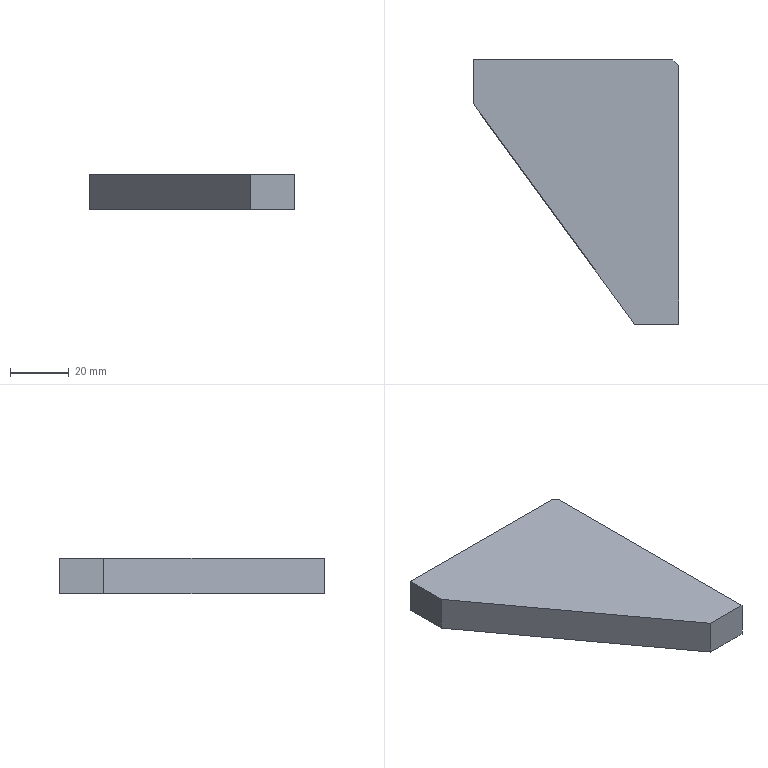Part | SolidWorks | features HoleWzd 2, Chamfer 1, Extrusion 1 | 1 solid | 24 faces | box 70 x 90 x 12 mm | volume 50116 mm3 | cylinder 8 | cone 8 | plane 8 | commonest cylinder face diameters 4.2 x8
STEP:
#1=CARTESIAN_POINT('',(-12.4,-75.,8.1));
#2=VERTEX_POINT('',#1);
#3=CARTESIAN_POINT('',(-12.4,-75.,3.9));
#4=VERTEX_POINT('',#3);
#5=CARTESIAN_POINT('',(-12.4,-75.,6.));
#6=DIRECTION('',(1.,0.,0.));
#7=DIRECTION('',(0.,0.,-1.));
#8=AXIS2_PLACEMENT_3D('',#5,#6,#7);
#9=CIRCLE('',#8,2.1);
#10=EDGE_CURVE('',#2,#4,#9,.T.);
#11=ORIENTED_EDGE('',*,*,#10,.F.);
#12=CARTESIAN_POINT('',(0.,-75.,8.1));
#13=VERTEX_POINT('',#12);
#14=CARTESIAN_POINT('',(0.,-75.,8.1));
#15=DIRECTION('',(1.,0.,0.));
#16=VECTOR('',#15,1000.);
#17=LINE('',#14,#16);
#18=EDGE_CURVE('',#2,#13,#17,.T.);
#19=ORIENTED_EDGE('',*,*,#18,.T.);
#20=CARTESIAN_POINT('',(0.,-75.,3.9));
#21=VERTEX_POINT('',#20);
#22=CARTESIAN_POINT('',(0.,-75.,6.));
#23=DIRECTION('',(1.,0.,0.));
#24=DIRECTION('',(0.,0.,-1.));
#25=AXIS2_PLACEMENT_3D('',#22,#23,#24);
#26=CIRCLE('',#25,2.1);
#27=EDGE_CURVE('',#13,#21,#26,.T.);
#28=ORIENTED_EDGE('',*,*,#27,.T.);
#29=CARTESIAN_POINT('',(0.,-75.,3.9));
#30=DIRECTION('',(1.,0.,0.));
#31=VECTOR('',#30,1000.);
#32=LINE('',#29,#31);
#33=EDGE_CURVE('',#4,#21,#32,.T.);
#34=ORIENTED_EDGE('',*,*,#33,.F.);
#35=EDGE_LOOP('',(#11,#19,#28,#34));
#36=FACE_OUTER_BOUND('',#35,.T.);
#37=CARTESIAN_POINT('',(0.,-75.,6.));
#38=DIRECTION('',(1.,0.,0.));
#39=DIRECTION('',(0.,0.,-1.));
#40=AXIS2_PLACEMENT_3D('',#37,#38,#39);
#41=CYLINDRICAL_SURFACE('',#40,2.1);
#42=ADVANCED_FACE('',(#36),#41,.F.);
#43=CARTESIAN_POINT('',(-13.662,-75.,6.));
#44=VERTEX_POINT('',#43);
#45=CARTESIAN_POINT('',(-12.4,-75.,3.9));
#46=DIRECTION('',(0.515,0.,-0.8572));
#47=VECTOR('',#46,1000.);
#48=LINE('',#45,#47);
#49=EDGE_CURVE('',#44,#4,#48,.T.);
#50=ORIENTED_EDGE('',*,*,#49,.F.);
#51=CARTESIAN_POINT('',(-12.4,-75.,8.1));
#52=DIRECTION('',(0.515,0.,0.8572));
#53=VECTOR('',#52,1000.);
#54=LINE('',#51,#53);
#55=EDGE_CURVE('',#44,#2,#54,.T.);
#56=ORIENTED_EDGE('',*,*,#55,.T.);
#57=ORIENTED_EDGE('',*,*,#10,.T.);
#58=EDGE_LOOP('',(#50,#56,#57));
#59=FACE_OUTER_BOUND('',#58,.T.);
#60=CARTESIAN_POINT('',(-12.4,-75.,6.));
#61=DIRECTION('',(1.,0.,0.));
#62=DIRECTION('',(0.,0.,-1.));
#63=AXIS2_PLACEMENT_3D('',#60,#61,#62);
#64=CONICAL_SURFACE('',#63,2.1,1.03);
#65=ADVANCED_FACE('',(#59),#64,.F.);
#66=CARTESIAN_POINT('',(-12.4,-25.,8.1));
#67=VERTEX_POINT('',#66);
#68=CARTESIAN_POINT('',(-12.4,-25.,3.9));
#69=VERTEX_POINT('',#68);
#70=CARTESIAN_POINT('',(-12.4,-25.,6.));
#71=DIRECTION('',(1.,0.,0.));
#72=DIRECTION('',(0.,0.,-1.));
#73=AXIS2_PLACEMENT_3D('',#70,#71,#72);
#74=CIRCLE('',#73,2.1);
#75=EDGE_CURVE('',#67,#69,#74,.T.);
#76=ORIENTED_EDGE('',*,*,#75,.F.);
#77=CARTESIAN_POINT('',(0.,-25.,8.1));
#78=VERTEX_POINT('',#77);
#79=CARTESIAN_POINT('',(0.,-25.,8.1));
#80=DIRECTION('',(1.,0.,0.));
#81=VECTOR('',#80,1000.);
#82=LINE('',#79,#81);
#83=EDGE_CURVE('',#67,#78,#82,.T.);
#84=ORIENTED_EDGE('',*,*,#83,.T.);
#85=CARTESIAN_POINT('',(0.,-25.,3.9));
#86=VERTEX_POINT('',#85);
#87=CARTESIAN_POINT('',(0.,-25.,6.));
#88=DIRECTION('',(1.,0.,0.));
#89=DIRECTION('',(0.,0.,-1.));
#90=AXIS2_PLACEMENT_3D('',#87,#88,#89);
#91=CIRCLE('',#90,2.1);
#92=EDGE_CURVE('',#78,#86,#91,.T.);
#93=ORIENTED_EDGE('',*,*,#92,.T.);
#94=CARTESIAN_POINT('',(0.,-25.,3.9));
#95=DIRECTION('',(1.,0.,0.));
#96=VECTOR('',#95,1000.);
#97=LINE('',#94,#96);
#98=EDGE_CURVE('',#69,#86,#97,.T.);
#99=ORIENTED_EDGE('',*,*,#98,.F.);
#100=EDGE_LOOP('',(#76,#84,#93,#99));
#101=FACE_OUTER_BOUND('',#100,.T.);
#102=CARTESIAN_POINT('',(0.,-25.,6.));
#103=DIRECTION('',(1.,0.,0.));
#104=DIRECTION('',(0.,0.,-1.));
#105=AXIS2_PLACEMENT_3D('',#102,#103,#104);
#106=CYLINDRICAL_SURFACE('',#105,2.1);
#107=ADVANCED_FACE('',(#101),#106,.F.);
#108=CARTESIAN_POINT('',(-13.662,-25.,6.));
#109=VERTEX_POINT('',#108);
#110=CARTESIAN_POINT('',(-12.4,-25.,3.9));
#111=DIRECTION('',(0.515,0.,-0.8572));
#112=VECTOR('',#111,1000.);
#113=LINE('',#110,#112);
#114=EDGE_CURVE('',#109,#69,#113,.T.);
#115=ORIENTED_EDGE('',*,*,#114,.F.);
#116=CARTESIAN_POINT('',(-12.4,-25.,8.1));
#117=DIRECTION('',(0.515,0.,0.8572));
#118=VECTOR('',#117,1000.);
#119=LINE('',#116,#118);
#120=EDGE_CURVE('',#109,#67,#119,.T.);
#121=ORIENTED_EDGE('',*,*,#120,.T.);
#122=ORIENTED_EDGE('',*,*,#75,.T.);
#123=EDGE_LOOP('',(#115,#121,#122));
#124=FACE_OUTER_BOUND('',#123,.T.);
#125=CARTESIAN_POINT('',(-12.4,-25.,6.));
#126=DIRECTION('',(1.,0.,0.));
#127=DIRECTION('',(0.,0.,-1.));
#128=AXIS2_PLACEMENT_3D('',#125,#126,#127);
#129=CONICAL_SURFACE('',#128,2.1,1.03);
#130=ADVANCED_FACE('',(#124),#129,.F.);
#131=CARTESIAN_POINT('',(-60.,-12.4,3.9));
#132=VERTEX_POINT('',#131);
#133=CARTESIAN_POINT('',(-60.,-12.4,8.1));
#134=VERTEX_POINT('',#133);
#135=CARTESIAN_POINT('',(-60.,-12.4,6.));
#136=DIRECTION('',(0.,1.,0.));
#137=DIRECTION('',(0.,0.,1.));
#138=AXIS2_PLACEMENT_3D('',#135,#136,#137);
#139=CIRCLE('',#138,2.1);
#140=EDGE_CURVE('',#132,#134,#139,.T.);
#141=ORIENTED_EDGE('',*,*,#140,.F.);
#142=CARTESIAN_POINT('',(-60.,0.,3.9));
#143=VERTEX_POINT('',#142);
#144=CARTESIAN_POINT('',(-60.,0.,3.9));
#145=DIRECTION('',(0.,1.,0.));
#146=VECTOR('',#145,1000.);
#147=LINE('',#144,#146);
#148=EDGE_CURVE('',#132,#143,#147,.T.);
#149=ORIENTED_EDGE('',*,*,#148,.T.);
#150=CARTESIAN_POINT('',(-60.,0.,8.1));
#151=VERTEX_POINT('',#150);
#152=CARTESIAN_POINT('',(-60.,0.,6.));
#153=DIRECTION('',(0.,1.,0.));
#154=DIRECTION('',(0.,0.,1.));
#155=AXIS2_PLACEMENT_3D('',#152,#153,#154);
#156=CIRCLE('',#155,2.1);
#157=EDGE_CURVE('',#143,#151,#156,.T.);
#158=ORIENTED_EDGE('',*,*,#157,.T.);
#159=CARTESIAN_POINT('',(-60.,0.,8.1));
#160=DIRECTION('',(0.,1.,0.));
#161=VECTOR('',#160,1000.);
#162=LINE('',#159,#161);
#163=EDGE_CURVE('',#134,#151,#162,.T.);
#164=ORIENTED_EDGE('',*,*,#163,.F.);
#165=EDGE_LOOP('',(#141,#149,#158,#164));
#166=FACE_OUTER_BOUND('',#165,.T.);
#167=CARTESIAN_POINT('',(-60.,0.,6.));
#168=DIRECTION('',(0.,1.,0.));
#169=DIRECTION('',(0.,0.,1.));
#170=AXIS2_PLACEMENT_3D('',#167,#168,#169);
#171=CYLINDRICAL_SURFACE('',#170,2.1);
#172=ADVANCED_FACE('',(#166),#171,.F.);
#173=CARTESIAN_POINT('',(-60.,-13.662,6.));
#174=VERTEX_POINT('',#173);
#175=CARTESIAN_POINT('',(-60.,-12.4,8.1));
#176=DIRECTION('',(0.,0.515,0.8572));
#177=VECTOR('',#176,1000.);
#178=LINE('',#175,#177);
#179=EDGE_CURVE('',#174,#134,#178,.T.);
#180=ORIENTED_EDGE('',*,*,#179,.F.);
#181=CARTESIAN_POINT('',(-60.,-12.4,3.9));
#182=DIRECTION('',(0.,0.515,-0.8572));
#183=VECTOR('',#182,1000.);
#184=LINE('',#181,#183);
#185=EDGE_CURVE('',#174,#132,#184,.T.);
#186=ORIENTED_EDGE('',*,*,#185,.T.);
#187=ORIENTED_EDGE('',*,*,#140,.T.);
#188=EDGE_LOOP('',(#180,#186,#187));
#189=FACE_OUTER_BOUND('',#188,.T.);
#190=CARTESIAN_POINT('',(-60.,-12.4,6.));
#191=DIRECTION('',(0.,1.,0.));
#192=DIRECTION('',(0.,0.,1.));
#193=AXIS2_PLACEMENT_3D('',#190,#191,#192);
#194=CONICAL_SURFACE('',#193,2.1,1.03);
#195=ADVANCED_FACE('',(#189),#194,.F.);
#196=CARTESIAN_POINT('',(-30.,-12.4,3.9));
#197=VERTEX_POINT('',#196);
#198=CARTESIAN_POINT('',(-30.,-12.4,8.1));
#199=VERTEX_POINT('',#198);
#200=CARTESIAN_POINT('',(-30.,-12.4,6.));
#201=DIRECTION('',(0.,1.,0.));
#202=DIRECTION('',(0.,0.,1.));
#203=AXIS2_PLACEMENT_3D('',#200,#201,#202);
#204=CIRCLE('',#203,2.1);
#205=EDGE_CURVE('',#197,#199,#204,.T.);
#206=ORIENTED_EDGE('',*,*,#205,.F.);
#207=CARTESIAN_POINT('',(-30.,0.,3.9));
#208=VERTEX_POINT('',#207);
#209=CARTESIAN_POINT('',(-30.,0.,3.9));
#210=DIRECTION('',(0.,1.,0.));
#211=VECTOR('',#210,1000.);
#212=LINE('',#209,#211);
#213=EDGE_CURVE('',#197,#208,#212,.T.);
#214=ORIENTED_EDGE('',*,*,#213,.T.);
#215=CARTESIAN_POINT('',(-30.,0.,8.1));
#216=VERTEX_POINT('',#215);
#217=CARTESIAN_POINT('',(-30.,0.,6.));
#218=DIRECTION('',(0.,1.,0.));
#219=DIRECTION('',(0.,0.,1.));
#220=AXIS2_PLACEMENT_3D('',#217,#218,#219);
#221=CIRCLE('',#220,2.1);
#222=EDGE_CURVE('',#208,#216,#221,.T.);
#223=ORIENTED_EDGE('',*,*,#222,.T.);
#224=CARTESIAN_POINT('',(-30.,0.,8.1));
#225=DIRECTION('',(0.,1.,0.));
#226=VECTOR('',#225,1000.);
#227=LINE('',#224,#226);
#228=EDGE_CURVE('',#199,#216,#227,.T.);
#229=ORIENTED_EDGE('',*,*,#228,.F.);
#230=EDGE_LOOP('',(#206,#214,#223,#229));
#231=FACE_OUTER_BOUND('',#230,.T.);
#232=CARTESIAN_POINT('',(-30.,0.,6.));
#233=DIRECTION('',(0.,1.,0.));
#234=DIRECTION('',(0.,0.,1.));
#235=AXIS2_PLACEMENT_3D('',#232,#233,#234);
#236=CYLINDRICAL_SURFACE('',#235,2.1);
#237=ADVANCED_FACE('',(#231),#236,.F.);
#238=CARTESIAN_POINT('',(-30.,-13.662,6.));
#239=VERTEX_POINT('',#238);
#240=CARTESIAN_POINT('',(-30.,-12.4,8.1));
#241=DIRECTION('',(0.,0.515,0.8572));
#242=VECTOR('',#241,1000.);
#243=LINE('',#240,#242);
#244=EDGE_CURVE('',#239,#199,#243,.T.);
#245=ORIENTED_EDGE('',*,*,#244,.F.);
#246=CARTESIAN_POINT('',(-30.,-12.4,3.9));
#247=DIRECTION('',(0.,0.515,-0.8572));
#248=VECTOR('',#247,1000.);
#249=LINE('',#246,#248);
#250=EDGE_CURVE('',#239,#197,#249,.T.);
#251=ORIENTED_EDGE('',*,*,#250,.T.);
#252=ORIENTED_EDGE('',*,*,#205,.T.);
#253=EDGE_LOOP('',(#245,#251,#252));
#254=FACE_OUTER_BOUND('',#253,.T.);
#255=CARTESIAN_POINT('',(-30.,-12.4,6.));
#256=DIRECTION('',(0.,1.,0.));
#257=DIRECTION('',(0.,0.,1.));
#258=AXIS2_PLACEMENT_3D('',#255,#256,#257);
#259=CONICAL_SURFACE('',#258,2.1,1.03);
#260=ADVANCED_FACE('',(#254),#259,.F.);
#261=CARTESIAN_POINT('',(-60.,0.,6.));
#262=DIRECTION('',(0.,1.,0.));
#263=DIRECTION('',(0.,0.,1.));
#264=AXIS2_PLACEMENT_3D('',#261,#262,#263);
#265=CIRCLE('',#264,2.1);
#266=EDGE_CURVE('',#151,#143,#265,.T.);
#267=ORIENTED_EDGE('',*,*,#266,.F.);
#268=ORIENTED_EDGE('',*,*,#157,.F.);
#269=EDGE_LOOP('',(#267,#268));
#270=FACE_BOUND('',#269,.T.);
#271=CARTESIAN_POINT('',(-30.,0.,6.));
#272=DIRECTION('',(0.,1.,0.));
#273=DIRECTION('',(0.,0.,1.));
#274=AXIS2_PLACEMENT_3D('',#271,#272,#273);
#275=CIRCLE('',#274,2.1);
#276=EDGE_CURVE('',#216,#208,#275,.T.);
#277=ORIENTED_EDGE('',*,*,#276,.F.);
#278=ORIENTED_EDGE('',*,*,#222,.F.);
#279=EDGE_LOOP('',(#277,#278));
#280=FACE_BOUND('',#279,.T.);
#281=CARTESIAN_POINT('',(-2.,0.,12.));
#282=VERTEX_POINT('',#281);
#283=CARTESIAN_POINT('',(-70.,0.,12.));
#284=VERTEX_POINT('',#283);
#285=CARTESIAN_POINT('',(-70.,0.,12.));
#286=DIRECTION('',(-1.,0.,0.));
#287=VECTOR('',#286,1000.);
#288=LINE('',#285,#287);
#289=EDGE_CURVE('',#282,#284,#288,.T.);
#290=ORIENTED_EDGE('',*,*,#289,.F.);
#291=CARTESIAN_POINT('',(-2.,0.,0.));
#292=VERTEX_POINT('',#291);
#293=CARTESIAN_POINT('',(-2.,0.,12.));
#294=DIRECTION('',(0.,0.,-1.));
#295=VECTOR('',#294,1000.);
#296=LINE('',#293,#295);
#297=EDGE_CURVE('',#282,#292,#296,.T.);
#298=ORIENTED_EDGE('',*,*,#297,.T.);
#299=CARTESIAN_POINT('',(-70.,0.,0.));
#300=VERTEX_POINT('',#299);
#301=CARTESIAN_POINT('',(-70.,0.,0.));
#302=DIRECTION('',(-1.,0.,0.));
#303=VECTOR('',#302,1000.);
#304=LINE('',#301,#303);
#305=EDGE_CURVE('',#292,#300,#304,.T.);
#306=ORIENTED_EDGE('',*,*,#305,.T.);
#307=CARTESIAN_POINT('',(-70.,0.,12.));
#308=DIRECTION('',(0.,0.,-1.));
#309=VECTOR('',#308,1000.);
#310=LINE('',#307,#309);
#311=EDGE_CURVE('',#284,#300,#310,.T.);
#312=ORIENTED_EDGE('',*,*,#311,.F.);
#313=EDGE_LOOP('',(#290,#298,#306,#312));
#314=FACE_OUTER_BOUND('',#313,.T.);
#315=CARTESIAN_POINT('',(-70.,0.,12.));
#316=DIRECTION('',(0.,-1.,0.));
#317=DIRECTION('',(0.,0.,-1.));
#318=AXIS2_PLACEMENT_3D('',#315,#316,#317);
#319=PLANE('',#318);
#320=ADVANCED_FACE('',(#270,#280,#314),#319,.F.);
#321=CARTESIAN_POINT('',(-70.,-15.,0.));
#322=VERTEX_POINT('',#321);
#323=CARTESIAN_POINT('',(-70.,-15.,0.));
#324=DIRECTION('',(0.,-1.,0.));
#325=VECTOR('',#324,1000.);
#326=LINE('',#323,#325);
#327=EDGE_CURVE('',#300,#322,#326,.T.);
#328=ORIENTED_EDGE('',*,*,#327,.T.);
#329=CARTESIAN_POINT('',(-70.,-15.,12.));
#330=VERTEX_POINT('',#329);
#331=CARTESIAN_POINT('',(-70.,-15.,12.));
#332=DIRECTION('',(0.,0.,-1.));
#333=VECTOR('',#332,1000.);
#334=LINE('',#331,#333);
#335=EDGE_CURVE('',#330,#322,#334,.T.);
#336=ORIENTED_EDGE('',*,*,#335,.F.);
#337=CARTESIAN_POINT('',(-70.,-15.,12.));
#338=DIRECTION('',(0.,-1.,0.));
#339=VECTOR('',#338,1000.);
#340=LINE('',#337,#339);
#341=EDGE_CURVE('',#284,#330,#340,.T.);
#342=ORIENTED_EDGE('',*,*,#341,.F.);
#343=ORIENTED_EDGE('',*,*,#311,.T.);
#344=EDGE_LOOP('',(#328,#336,#342,#343));
#345=FACE_OUTER_BOUND('',#344,.T.);
#346=CARTESIAN_POINT('',(-70.,-15.,12.));
#347=DIRECTION('',(1.,0.,0.));
#348=DIRECTION('',(0.,0.,-1.));
#349=AXIS2_PLACEMENT_3D('',#346,#347,#348);
#350=PLANE('',#349);
#351=ADVANCED_FACE('',(#345),#350,.F.);
#352=CARTESIAN_POINT('',(-15.,-90.,0.));
#353=VERTEX_POINT('',#352);
#354=CARTESIAN_POINT('',(-15.,-90.,0.));
#355=DIRECTION('',(0.5914,-0.8064,0.));
#356=VECTOR('',#355,1000.);
#357=LINE('',#354,#356);
#358=EDGE_CURVE('',#322,#353,#357,.T.);
#359=ORIENTED_EDGE('',*,*,#358,.T.);
#360=CARTESIAN_POINT('',(-15.,-90.,12.));
#361=VERTEX_POINT('',#360);
#362=CARTESIAN_POINT('',(-15.,-90.,12.));
#363=DIRECTION('',(0.,0.,-1.));
#364=VECTOR('',#363,1000.);
#365=LINE('',#362,#364);
#366=EDGE_CURVE('',#361,#353,#365,.T.);
#367=ORIENTED_EDGE('',*,*,#366,.F.);
#368=CARTESIAN_POINT('',(-15.,-90.,12.));
#369=DIRECTION('',(0.5914,-0.8064,0.));
#370=VECTOR('',#369,1000.);
#371=LINE('',#368,#370);
#372=EDGE_CURVE('',#330,#361,#371,.T.);
#373=ORIENTED_EDGE('',*,*,#372,.F.);
#374=ORIENTED_EDGE('',*,*,#335,.T.);
#375=EDGE_LOOP('',(#359,#367,#373,#374));
#376=FACE_OUTER_BOUND('',#375,.T.);
#377=CARTESIAN_POINT('',(-15.,-90.,12.));
#378=DIRECTION('',(0.8064,0.5914,0.));
#379=DIRECTION('',(-0.5914,0.8064,0.));
#380=AXIS2_PLACEMENT_3D('',#377,#378,#379);
#381=PLANE('',#380);
#382=ADVANCED_FACE('',(#376),#381,.F.);
#383=CARTESIAN_POINT('',(0.,-90.,0.));
#384=VERTEX_POINT('',#383);
#385=CARTESIAN_POINT('',(0.,-90.,0.));
#386=DIRECTION('',(1.,0.,0.));
#387=VECTOR('',#386,1000.);
#388=LINE('',#385,#387);
#389=EDGE_CURVE('',#353,#384,#388,.T.);
#390=ORIENTED_EDGE('',*,*,#389,.T.);
#391=CARTESIAN_POINT('',(0.,-90.,12.));
#392=VERTEX_POINT('',#391);
#393=CARTESIAN_POINT('',(0.,-90.,12.));
#394=DIRECTION('',(0.,0.,-1.));
#395=VECTOR('',#394,1000.);
#396=LINE('',#393,#395);
#397=EDGE_CURVE('',#392,#384,#396,.T.);
#398=ORIENTED_EDGE('',*,*,#397,.F.);
#399=CARTESIAN_POINT('',(0.,-90.,12.));
#400=DIRECTION('',(1.,0.,0.));
#401=VECTOR('',#400,1000.);
#402=LINE('',#399,#401);
#403=EDGE_CURVE('',#361,#392,#402,.T.);
#404=ORIENTED_EDGE('',*,*,#403,.F.);
#405=ORIENTED_EDGE('',*,*,#366,.T.);
#406=EDGE_LOOP('',(#390,#398,#404,#405));
#407=FACE_OUTER_BOUND('',#406,.T.);
#408=CARTESIAN_POINT('',(0.,-90.,12.));
#409=DIRECTION('',(0.,1.,0.));
#410=DIRECTION('',(0.,0.,1.));
#411=AXIS2_PLACEMENT_3D('',#408,#409,#410);
#412=PLANE('',#411);
#413=ADVANCED_FACE('',(#407),#412,.F.);
#414=CARTESIAN_POINT('',(0.,-75.,6.));
#415=DIRECTION('',(1.,0.,0.));
#416=DIRECTION('',(0.,0.,-1.));
#417=AXIS2_PLACEMENT_3D('',#414,#415,#416);
#418=CIRCLE('',#417,2.1);
#419=EDGE_CURVE('',#21,#13,#418,.T.);
#420=ORIENTED_EDGE('',*,*,#419,.F.);
#421=ORIENTED_EDGE('',*,*,#27,.F.);
#422=EDGE_LOOP('',(#420,#421));
#423=FACE_BOUND('',#422,.T.);
#424=CARTESIAN_POINT('',(0.,-25.,6.));
#425=DIRECTION('',(1.,0.,0.));
#426=DIRECTION('',(0.,0.,-1.));
#427=AXIS2_PLACEMENT_3D('',#424,#425,#426);
#428=CIRCLE('',#427,2.1);
#429=EDGE_CURVE('',#86,#78,#428,.T.);
#430=ORIENTED_EDGE('',*,*,#429,.F.);
#431=ORIENTED_EDGE('',*,*,#92,.F.);
#432=EDGE_LOOP('',(#430,#431));
#433=FACE_BOUND('',#432,.T.);
#434=CARTESIAN_POINT('',(0.,-2.,0.));
#435=VERTEX_POINT('',#434);
#436=CARTESIAN_POINT('',(0.,0.,0.));
#437=DIRECTION('',(0.,1.,0.));
#438=VECTOR('',#437,1000.);
#439=LINE('',#436,#438);
#440=EDGE_CURVE('',#384,#435,#439,.T.);
#441=ORIENTED_EDGE('',*,*,#440,.T.);
#442=CARTESIAN_POINT('',(0.,-2.,12.));
#443=VERTEX_POINT('',#442);
#444=CARTESIAN_POINT('',(0.,-2.,12.));
#445=DIRECTION('',(0.,0.,1.));
#446=VECTOR('',#445,1000.);
#447=LINE('',#444,#446);
#448=EDGE_CURVE('',#435,#443,#447,.T.);
#449=ORIENTED_EDGE('',*,*,#448,.T.);
#450=CARTESIAN_POINT('',(0.,0.,12.));
#451=DIRECTION('',(0.,1.,0.));
#452=VECTOR('',#451,1000.);
#453=LINE('',#450,#452);
#454=EDGE_CURVE('',#392,#443,#453,.T.);
#455=ORIENTED_EDGE('',*,*,#454,.F.);
#456=ORIENTED_EDGE('',*,*,#397,.T.);
#457=EDGE_LOOP('',(#441,#449,#455,#456));
#458=FACE_OUTER_BOUND('',#457,.T.);
#459=CARTESIAN_POINT('',(0.,0.,12.));
#460=DIRECTION('',(-1.,0.,0.));
#461=DIRECTION('',(0.,-1.,0.));
#462=AXIS2_PLACEMENT_3D('',#459,#460,#461);
#463=PLANE('',#462);
#464=ADVANCED_FACE('',(#423,#433,#458),#463,.F.);
#465=ORIENTED_EDGE('',*,*,#454,.T.);
#466=CARTESIAN_POINT('',(-2.,0.,12.));
#467=DIRECTION('',(-0.7071,0.7071,0.));
#468=VECTOR('',#467,1000.);
#469=LINE('',#466,#468);
#470=EDGE_CURVE('',#443,#282,#469,.T.);
#471=ORIENTED_EDGE('',*,*,#470,.T.);
#472=ORIENTED_EDGE('',*,*,#289,.T.);
#473=ORIENTED_EDGE('',*,*,#341,.T.);
#474=ORIENTED_EDGE('',*,*,#372,.T.);
#475=ORIENTED_EDGE('',*,*,#403,.T.);
#476=EDGE_LOOP('',(#465,#471,#472,#473,#474,#475));
#477=FACE_OUTER_BOUND('',#476,.T.);
#478=CARTESIAN_POINT('',(0.,0.,12.));
#479=DIRECTION('',(0.,0.,-1.));
#480=DIRECTION('',(-1.,0.,0.));
#481=AXIS2_PLACEMENT_3D('',#478,#479,#480);
#482=PLANE('',#481);
#483=ADVANCED_FACE('',(#477),#482,.F.);
#484=ORIENTED_EDGE('',*,*,#305,.F.);
#485=CARTESIAN_POINT('',(-1.,-1.,0.));
#486=DIRECTION('',(0.7071,-0.7071,0.));
#487=VECTOR('',#486,1000.);
#488=LINE('',#485,#487);
#489=EDGE_CURVE('',#292,#435,#488,.T.);
#490=ORIENTED_EDGE('',*,*,#489,.T.);
#491=ORIENTED_EDGE('',*,*,#440,.F.);
#492=ORIENTED_EDGE('',*,*,#389,.F.);
#493=ORIENTED_EDGE('',*,*,#358,.F.);
#494=ORIENTED_EDGE('',*,*,#327,.F.);
#495=EDGE_LOOP('',(#484,#490,#491,#492,#493,#494));
#496=FACE_OUTER_BOUND('',#495,.T.);
#497=CARTESIAN_POINT('',(0.,0.,0.));
#498=DIRECTION('',(0.,0.,-1.));
#499=DIRECTION('',(-1.,0.,0.));
#500=AXIS2_PLACEMENT_3D('',#497,#498,#499);
#501=PLANE('',#500);
#502=ADVANCED_FACE('',(#496),#501,.T.);
#503=ORIENTED_EDGE('',*,*,#250,.F.);
#504=ORIENTED_EDGE('',*,*,#244,.T.);
#505=CARTESIAN_POINT('',(-30.,-12.4,6.));
#506=DIRECTION('',(0.,1.,0.));
#507=DIRECTION('',(0.,0.,1.));
#508=AXIS2_PLACEMENT_3D('',#505,#506,#507);
#509=CIRCLE('',#508,2.1);
#510=EDGE_CURVE('',#199,#197,#509,.T.);
#511=ORIENTED_EDGE('',*,*,#510,.T.);
#512=EDGE_LOOP('',(#503,#504,#511));
#513=FACE_OUTER_BOUND('',#512,.T.);
#514=CARTESIAN_POINT('',(-30.,-12.4,6.));
#515=DIRECTION('',(0.,1.,0.));
#516=DIRECTION('',(0.,0.,1.));
#517=AXIS2_PLACEMENT_3D('',#514,#515,#516);
#518=CONICAL_SURFACE('',#517,2.1,1.03);
#519=ADVANCED_FACE('',(#513),#518,.F.);
#520=ORIENTED_EDGE('',*,*,#213,.F.);
#521=ORIENTED_EDGE('',*,*,#510,.F.);
#522=ORIENTED_EDGE('',*,*,#228,.T.);
#523=ORIENTED_EDGE('',*,*,#276,.T.);
#524=EDGE_LOOP('',(#520,#521,#522,#523));
#525=FACE_OUTER_BOUND('',#524,.T.);
#526=CARTESIAN_POINT('',(-30.,0.,6.));
#527=DIRECTION('',(0.,1.,0.));
#528=DIRECTION('',(0.,0.,1.));
#529=AXIS2_PLACEMENT_3D('',#526,#527,#528);
#530=CYLINDRICAL_SURFACE('',#529,2.1);
#531=ADVANCED_FACE('',(#525),#530,.F.);
#532=ORIENTED_EDGE('',*,*,#185,.F.);
#533=ORIENTED_EDGE('',*,*,#179,.T.);
#534=CARTESIAN_POINT('',(-60.,-12.4,6.));
#535=DIRECTION('',(0.,1.,0.));
#536=DIRECTION('',(0.,0.,1.));
#537=AXIS2_PLACEMENT_3D('',#534,#535,#536);
#538=CIRCLE('',#537,2.1);
#539=EDGE_CURVE('',#134,#132,#538,.T.);
#540=ORIENTED_EDGE('',*,*,#539,.T.);
#541=EDGE_LOOP('',(#532,#533,#540));
#542=FACE_OUTER_BOUND('',#541,.T.);
#543=CARTESIAN_POINT('',(-60.,-12.4,6.));
#544=DIRECTION('',(0.,1.,0.));
#545=DIRECTION('',(0.,0.,1.));
#546=AXIS2_PLACEMENT_3D('',#543,#544,#545);
#547=CONICAL_SURFACE('',#546,2.1,1.03);
#548=ADVANCED_FACE('',(#542),#547,.F.);
#549=ORIENTED_EDGE('',*,*,#148,.F.);
#550=ORIENTED_EDGE('',*,*,#539,.F.);
#551=ORIENTED_EDGE('',*,*,#163,.T.);
#552=ORIENTED_EDGE('',*,*,#266,.T.);
#553=EDGE_LOOP('',(#549,#550,#551,#552));
#554=FACE_OUTER_BOUND('',#553,.T.);
#555=CARTESIAN_POINT('',(-60.,0.,6.));
#556=DIRECTION('',(0.,1.,0.));
#557=DIRECTION('',(0.,0.,1.));
#558=AXIS2_PLACEMENT_3D('',#555,#556,#557);
#559=CYLINDRICAL_SURFACE('',#558,2.1);
#560=ADVANCED_FACE('',(#554),#559,.F.);
#561=ORIENTED_EDGE('',*,*,#120,.F.);
#562=ORIENTED_EDGE('',*,*,#114,.T.);
#563=CARTESIAN_POINT('',(-12.4,-25.,6.));
#564=DIRECTION('',(1.,0.,0.));
#565=DIRECTION('',(0.,0.,-1.));
#566=AXIS2_PLACEMENT_3D('',#563,#564,#565);
#567=CIRCLE('',#566,2.1);
#568=EDGE_CURVE('',#69,#67,#567,.T.);
#569=ORIENTED_EDGE('',*,*,#568,.T.);
#570=EDGE_LOOP('',(#561,#562,#569));
#571=FACE_OUTER_BOUND('',#570,.T.);
#572=CARTESIAN_POINT('',(-12.4,-25.,6.));
#573=DIRECTION('',(1.,0.,0.));
#574=DIRECTION('',(0.,0.,-1.));
#575=AXIS2_PLACEMENT_3D('',#572,#573,#574);
#576=CONICAL_SURFACE('',#575,2.1,1.03);
#577=ADVANCED_FACE('',(#571),#576,.F.);
#578=ORIENTED_EDGE('',*,*,#83,.F.);
#579=ORIENTED_EDGE('',*,*,#568,.F.);
#580=ORIENTED_EDGE('',*,*,#98,.T.);
#581=ORIENTED_EDGE('',*,*,#429,.T.);
#582=EDGE_LOOP('',(#578,#579,#580,#581));
#583=FACE_OUTER_BOUND('',#582,.T.);
#584=CARTESIAN_POINT('',(0.,-25.,6.));
#585=DIRECTION('',(1.,0.,0.));
#586=DIRECTION('',(0.,0.,-1.));
#587=AXIS2_PLACEMENT_3D('',#584,#585,#586);
#588=CYLINDRICAL_SURFACE('',#587,2.1);
#589=ADVANCED_FACE('',(#583),#588,.F.);
#590=ORIENTED_EDGE('',*,*,#55,.F.);
#591=ORIENTED_EDGE('',*,*,#49,.T.);
#592=CARTESIAN_POINT('',(-12.4,-75.,6.));
#593=DIRECTION('',(1.,0.,0.));
#594=DIRECTION('',(0.,0.,-1.));
#595=AXIS2_PLACEMENT_3D('',#592,#593,#594);
#596=CIRCLE('',#595,2.1);
#597=EDGE_CURVE('',#4,#2,#596,.T.);
#598=ORIENTED_EDGE('',*,*,#597,.T.);
#599=EDGE_LOOP('',(#590,#591,#598));
#600=FACE_OUTER_BOUND('',#599,.T.);
#601=CARTESIAN_POINT('',(-12.4,-75.,6.));
#602=DIRECTION('',(1.,0.,0.));
#603=DIRECTION('',(0.,0.,-1.));
#604=AXIS2_PLACEMENT_3D('',#601,#602,#603);
#605=CONICAL_SURFACE('',#604,2.1,1.03);
#606=ADVANCED_FACE('',(#600),#605,.F.);
#607=ORIENTED_EDGE('',*,*,#18,.F.);
#608=ORIENTED_EDGE('',*,*,#597,.F.);
#609=ORIENTED_EDGE('',*,*,#33,.T.);
#610=ORIENTED_EDGE('',*,*,#419,.T.);
#611=EDGE_LOOP('',(#607,#608,#609,#610));
#612=FACE_OUTER_BOUND('',#611,.T.);
#613=CARTESIAN_POINT('',(0.,-75.,6.));
#614=DIRECTION('',(1.,0.,0.));
#615=DIRECTION('',(0.,0.,-1.));
#616=AXIS2_PLACEMENT_3D('',#613,#614,#615);
#617=CYLINDRICAL_SURFACE('',#616,2.1);
#618=ADVANCED_FACE('',(#612),#617,.F.);
#619=ORIENTED_EDGE('',*,*,#470,.F.);
#620=ORIENTED_EDGE('',*,*,#448,.F.);
#621=ORIENTED_EDGE('',*,*,#489,.F.);
#622=ORIENTED_EDGE('',*,*,#297,.F.);
#623=EDGE_LOOP('',(#619,#620,#621,#622));
#624=FACE_OUTER_BOUND('',#623,.T.);
#625=CARTESIAN_POINT('',(-2.,0.,12.));
#626=DIRECTION('',(-0.7071,-0.7071,0.));
#627=DIRECTION('',(0.,0.,-1.));
#628=AXIS2_PLACEMENT_3D('',#625,#626,#627);
#629=PLANE('',#628);
#630=ADVANCED_FACE('',(#624),#629,.F.);
#631=CLOSED_SHELL('',(#42,#65,#107,#130,#172,#195,#237,#260,#320,#351,#382,#413,#464,#483,#502,#519,#531,#548,#560,#577,#589,#606,#618,#630));
#632=MANIFOLD_SOLID_BREP('',#631);
#633=CARTESIAN_POINT('',(0.,0.,0.));
#634=DIRECTION('',(0.,0.,1.));
#635=DIRECTION('',(1.,0.,0.));
#636=AXIS2_PLACEMENT_3D('',#633,#634,#635);
#637=(LENGTH_UNIT()NAMED_UNIT(*)SI_UNIT(.MILLI.,.METRE.));
#638=UNCERTAINTY_MEASURE_WITH_UNIT(LENGTH_MEASURE(0.00001),#637,'','');
#639=(NAMED_UNIT(*)PLANE_ANGLE_UNIT()SI_UNIT($,.RADIAN.));
#640=(NAMED_UNIT(*)SI_UNIT($,.STERADIAN.)SOLID_ANGLE_UNIT());
#641=(GEOMETRIC_REPRESENTATION_CONTEXT(3)GLOBAL_UNCERTAINTY_ASSIGNED_CONTEXT((#638))GLOBAL_UNIT_ASSIGNED_CONTEXT((#637,#639,#640))REPRESENTATION_CONTEXT('',''));
#642=ADVANCED_BREP_SHAPE_REPRESENTATION('',(#632,#636),#641);